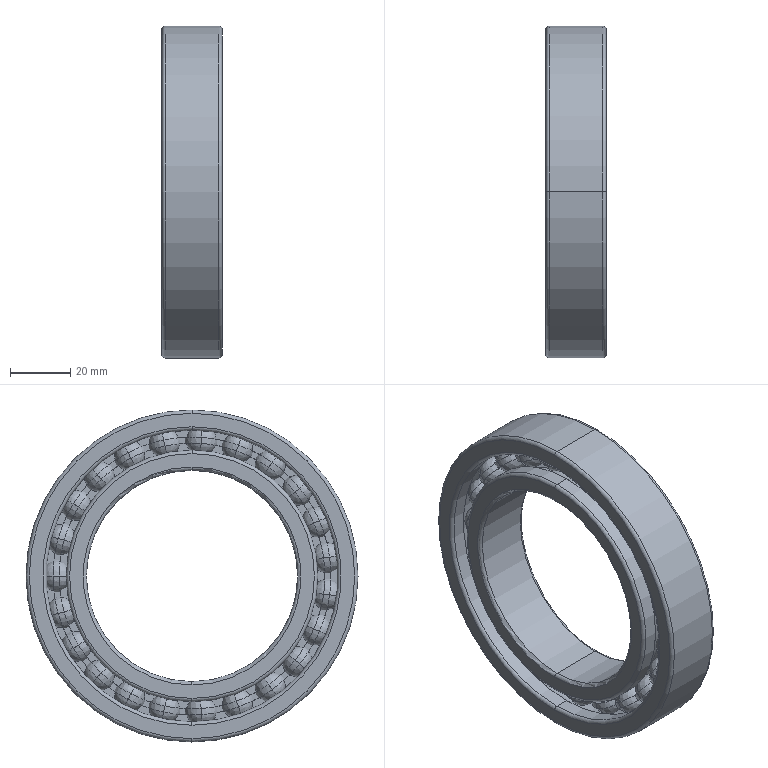Part | SolidWorks | features Revolution 5, CirPattern 2, RefAxis 1, RevCut 1 | 25 solids | 276 faces | box 20 x 110 x 110 mm | volume 84477 mm3 | cylinder 106 | sphere 96 | plane 52 | torus 20 | cone 2 | commonest cylinder face diameters 88 x45 92 x45 83.333 x4 96.667 x4 70 x2 78.889 x2